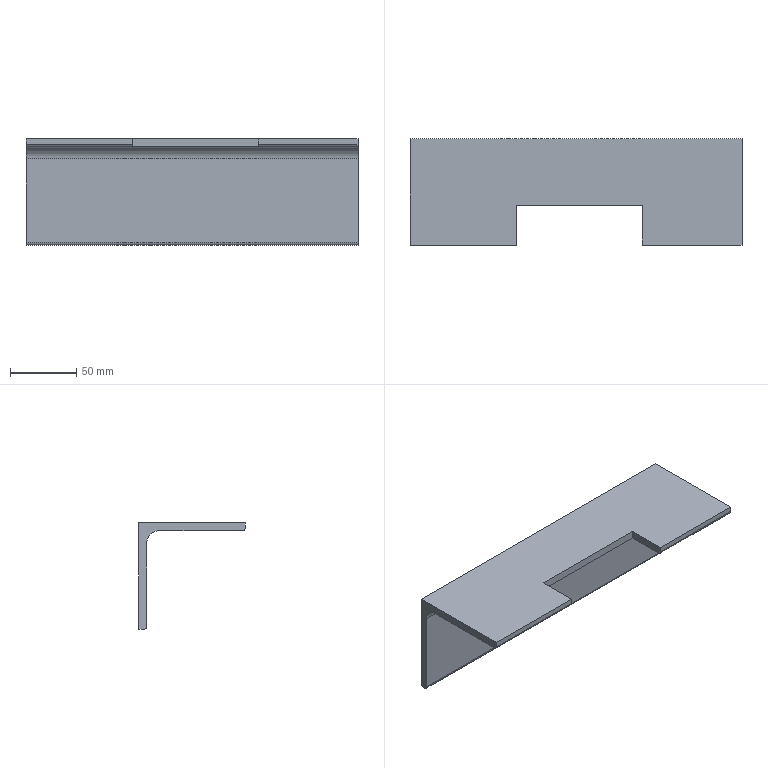Part | SolidWorks | features ICE 1, WeldMemberFeat 1, WeldmentFeature 1 | 1 solid | 16 faces | box 250 x 80 x 80 mm | volume 217898 mm3 | plane 12 | cylinder 4 | commonest cylinder face diameters 4 x3 18 x1
STEP:
#1=CARTESIAN_POINT('',(50.,-80.,0.));
#2=VERTEX_POINT('',#1);
#3=CARTESIAN_POINT('',(125.,-80.,0.));
#4=VERTEX_POINT('',#3);
#5=CARTESIAN_POINT('',(-125.,-80.,0.));
#6=DIRECTION('',(1.,0.,0.));
#7=VECTOR('',#6,1000.);
#8=LINE('',#5,#7);
#9=EDGE_CURVE('',#2,#4,#8,.T.);
#10=ORIENTED_EDGE('',*,*,#9,.F.);
#11=CARTESIAN_POINT('',(50.,-80.,-4.));
#12=VERTEX_POINT('',#11);
#13=CARTESIAN_POINT('',(50.,-80.,0.));
#14=DIRECTION('',(0.,0.,-1.));
#15=VECTOR('',#14,1000.);
#16=LINE('',#13,#15);
#17=EDGE_CURVE('',#2,#12,#16,.T.);
#18=ORIENTED_EDGE('',*,*,#17,.T.);
#19=CARTESIAN_POINT('',(125.,-80.,-4.));
#20=VERTEX_POINT('',#19);
#21=CARTESIAN_POINT('',(-125.,-80.,-4.));
#22=DIRECTION('',(1.,0.,0.));
#23=VECTOR('',#22,1000.);
#24=LINE('',#21,#23);
#25=EDGE_CURVE('',#12,#20,#24,.T.);
#26=ORIENTED_EDGE('',*,*,#25,.T.);
#27=CARTESIAN_POINT('',(125.,-80.,0.));
#28=DIRECTION('',(0.,0.,1.));
#29=VECTOR('',#28,1000.);
#30=LINE('',#27,#29);
#31=EDGE_CURVE('',#20,#4,#30,.T.);
#32=ORIENTED_EDGE('',*,*,#31,.T.);
#33=EDGE_LOOP('',(#10,#18,#26,#32));
#34=FACE_OUTER_BOUND('',#33,.T.);
#35=CARTESIAN_POINT('',(-125.,-80.,0.));
#36=DIRECTION('',(0.,1.,0.));
#37=DIRECTION('',(-1.,0.,0.));
#38=AXIS2_PLACEMENT_3D('',#35,#36,#37);
#39=PLANE('',#38);
#40=ADVANCED_FACE('',(#34),#39,.F.);
#41=ORIENTED_EDGE('',*,*,#25,.F.);
#42=CARTESIAN_POINT('',(50.,-78.,-6.));
#43=VERTEX_POINT('',#42);
#44=CARTESIAN_POINT('',(50.,-78.,-4.));
#45=DIRECTION('',(1.,0.,0.));
#46=DIRECTION('',(0.,1.,0.));
#47=AXIS2_PLACEMENT_3D('',#44,#45,#46);
#48=CIRCLE('',#47,2.);
#49=EDGE_CURVE('',#12,#43,#48,.T.);
#50=ORIENTED_EDGE('',*,*,#49,.T.);
#51=CARTESIAN_POINT('',(125.,-78.,-6.));
#52=VERTEX_POINT('',#51);
#53=CARTESIAN_POINT('',(-125.,-78.,-6.));
#54=DIRECTION('',(1.,0.,0.));
#55=VECTOR('',#54,1000.);
#56=LINE('',#53,#55);
#57=EDGE_CURVE('',#43,#52,#56,.T.);
#58=ORIENTED_EDGE('',*,*,#57,.T.);
#59=CARTESIAN_POINT('',(125.,-78.,-4.));
#60=DIRECTION('',(-1.,0.,0.));
#61=DIRECTION('',(0.,1.,0.));
#62=AXIS2_PLACEMENT_3D('',#59,#60,#61);
#63=CIRCLE('',#62,2.);
#64=EDGE_CURVE('',#52,#20,#63,.T.);
#65=ORIENTED_EDGE('',*,*,#64,.T.);
#66=EDGE_LOOP('',(#41,#50,#58,#65));
#67=FACE_OUTER_BOUND('',#66,.T.);
#68=CARTESIAN_POINT('',(-125.,-78.,-4.));
#69=DIRECTION('',(1.,0.,0.));
#70=DIRECTION('',(0.,1.,0.));
#71=AXIS2_PLACEMENT_3D('',#68,#69,#70);
#72=CYLINDRICAL_SURFACE('',#71,2.);
#73=ADVANCED_FACE('',(#67),#72,.T.);
#74=CARTESIAN_POINT('',(-125.,-80.,-4.));
#75=VERTEX_POINT('',#74);
#76=CARTESIAN_POINT('',(-45.,-80.,-4.));
#77=VERTEX_POINT('',#76);
#78=CARTESIAN_POINT('',(-125.,-80.,-4.));
#79=DIRECTION('',(1.,0.,0.));
#80=VECTOR('',#79,1000.);
#81=LINE('',#78,#80);
#82=EDGE_CURVE('',#75,#77,#81,.T.);
#83=ORIENTED_EDGE('',*,*,#82,.T.);
#84=CARTESIAN_POINT('',(-45.,-80.,0.));
#85=VERTEX_POINT('',#84);
#86=CARTESIAN_POINT('',(-45.,-80.,0.));
#87=DIRECTION('',(0.,0.,1.));
#88=VECTOR('',#87,1000.);
#89=LINE('',#86,#88);
#90=EDGE_CURVE('',#77,#85,#89,.T.);
#91=ORIENTED_EDGE('',*,*,#90,.T.);
#92=CARTESIAN_POINT('',(-125.,-80.,0.));
#93=VERTEX_POINT('',#92);
#94=CARTESIAN_POINT('',(-125.,-80.,0.));
#95=DIRECTION('',(1.,0.,0.));
#96=VECTOR('',#95,1000.);
#97=LINE('',#94,#96);
#98=EDGE_CURVE('',#93,#85,#97,.T.);
#99=ORIENTED_EDGE('',*,*,#98,.F.);
#100=CARTESIAN_POINT('',(-125.,-80.,0.));
#101=DIRECTION('',(0.,0.,1.));
#102=VECTOR('',#101,1000.);
#103=LINE('',#100,#102);
#104=EDGE_CURVE('',#75,#93,#103,.T.);
#105=ORIENTED_EDGE('',*,*,#104,.F.);
#106=EDGE_LOOP('',(#83,#91,#99,#105));
#107=FACE_OUTER_BOUND('',#106,.T.);
#108=CARTESIAN_POINT('',(-125.,-80.,0.));
#109=DIRECTION('',(0.,1.,0.));
#110=DIRECTION('',(-1.,0.,0.));
#111=AXIS2_PLACEMENT_3D('',#108,#109,#110);
#112=PLANE('',#111);
#113=ADVANCED_FACE('',(#107),#112,.F.);
#114=CARTESIAN_POINT('',(-45.,-50.,0.));
#115=VERTEX_POINT('',#114);
#116=CARTESIAN_POINT('',(50.,-50.,0.));
#117=VERTEX_POINT('',#116);
#118=CARTESIAN_POINT('',(-125.,-50.,0.));
#119=DIRECTION('',(1.,0.,0.));
#120=VECTOR('',#119,1000.);
#121=LINE('',#118,#120);
#122=EDGE_CURVE('',#115,#117,#121,.T.);
#123=ORIENTED_EDGE('',*,*,#122,.T.);
#124=CARTESIAN_POINT('',(50.,-80.,0.));
#125=DIRECTION('',(0.,-1.,0.));
#126=VECTOR('',#125,1000.);
#127=LINE('',#124,#126);
#128=EDGE_CURVE('',#117,#2,#127,.T.);
#129=ORIENTED_EDGE('',*,*,#128,.T.);
#130=ORIENTED_EDGE('',*,*,#9,.T.);
#131=CARTESIAN_POINT('',(125.,0.,0.));
#132=VERTEX_POINT('',#131);
#133=CARTESIAN_POINT('',(125.,-80.,0.));
#134=DIRECTION('',(0.,1.,0.));
#135=VECTOR('',#134,1000.);
#136=LINE('',#133,#135);
#137=EDGE_CURVE('',#4,#132,#136,.T.);
#138=ORIENTED_EDGE('',*,*,#137,.T.);
#139=CARTESIAN_POINT('',(-125.,0.,0.));
#140=VERTEX_POINT('',#139);
#141=CARTESIAN_POINT('',(-125.,0.,0.));
#142=DIRECTION('',(1.,0.,0.));
#143=VECTOR('',#142,1000.);
#144=LINE('',#141,#143);
#145=EDGE_CURVE('',#140,#132,#144,.T.);
#146=ORIENTED_EDGE('',*,*,#145,.F.);
#147=CARTESIAN_POINT('',(-125.,-80.,0.));
#148=DIRECTION('',(0.,1.,0.));
#149=VECTOR('',#148,1000.);
#150=LINE('',#147,#149);
#151=EDGE_CURVE('',#93,#140,#150,.T.);
#152=ORIENTED_EDGE('',*,*,#151,.F.);
#153=ORIENTED_EDGE('',*,*,#98,.T.);
#154=CARTESIAN_POINT('',(-45.,-80.,0.));
#155=DIRECTION('',(0.,1.,0.));
#156=VECTOR('',#155,1000.);
#157=LINE('',#154,#156);
#158=EDGE_CURVE('',#85,#115,#157,.T.);
#159=ORIENTED_EDGE('',*,*,#158,.T.);
#160=EDGE_LOOP('',(#123,#129,#130,#138,#146,#152,#153,#159));
#161=FACE_OUTER_BOUND('',#160,.T.);
#162=CARTESIAN_POINT('',(-125.,-80.,0.));
#163=DIRECTION('',(0.,0.,-1.));
#164=DIRECTION('',(0.,1.,0.));
#165=AXIS2_PLACEMENT_3D('',#162,#163,#164);
#166=PLANE('',#165);
#167=ADVANCED_FACE('',(#161),#166,.F.);
#168=CARTESIAN_POINT('',(125.,0.,-80.));
#169=VERTEX_POINT('',#168);
#170=CARTESIAN_POINT('',(125.,0.,0.));
#171=DIRECTION('',(0.,0.,-1.));
#172=VECTOR('',#171,1000.);
#173=LINE('',#170,#172);
#174=EDGE_CURVE('',#132,#169,#173,.T.);
#175=ORIENTED_EDGE('',*,*,#174,.T.);
#176=CARTESIAN_POINT('',(-125.,0.,-80.));
#177=VERTEX_POINT('',#176);
#178=CARTESIAN_POINT('',(-125.,0.,-80.));
#179=DIRECTION('',(1.,0.,0.));
#180=VECTOR('',#179,1000.);
#181=LINE('',#178,#180);
#182=EDGE_CURVE('',#177,#169,#181,.T.);
#183=ORIENTED_EDGE('',*,*,#182,.F.);
#184=CARTESIAN_POINT('',(-125.,0.,0.));
#185=DIRECTION('',(0.,0.,-1.));
#186=VECTOR('',#185,1000.);
#187=LINE('',#184,#186);
#188=EDGE_CURVE('',#140,#177,#187,.T.);
#189=ORIENTED_EDGE('',*,*,#188,.F.);
#190=ORIENTED_EDGE('',*,*,#145,.T.);
#191=EDGE_LOOP('',(#175,#183,#189,#190));
#192=FACE_OUTER_BOUND('',#191,.T.);
#193=CARTESIAN_POINT('',(-125.,0.,0.));
#194=DIRECTION('',(0.,-1.,0.));
#195=DIRECTION('',(1.,0.,0.));
#196=AXIS2_PLACEMENT_3D('',#193,#194,#195);
#197=PLANE('',#196);
#198=ADVANCED_FACE('',(#192),#197,.F.);
#199=CARTESIAN_POINT('',(125.,-4.,-80.));
#200=VERTEX_POINT('',#199);
#201=CARTESIAN_POINT('',(125.,0.,-80.));
#202=DIRECTION('',(0.,-1.,0.));
#203=VECTOR('',#202,1000.);
#204=LINE('',#201,#203);
#205=EDGE_CURVE('',#169,#200,#204,.T.);
#206=ORIENTED_EDGE('',*,*,#205,.T.);
#207=CARTESIAN_POINT('',(-125.,-4.,-80.));
#208=VERTEX_POINT('',#207);
#209=CARTESIAN_POINT('',(-125.,-4.,-80.));
#210=DIRECTION('',(1.,0.,0.));
#211=VECTOR('',#210,1000.);
#212=LINE('',#209,#211);
#213=EDGE_CURVE('',#208,#200,#212,.T.);
#214=ORIENTED_EDGE('',*,*,#213,.F.);
#215=CARTESIAN_POINT('',(-125.,0.,-80.));
#216=DIRECTION('',(0.,-1.,0.));
#217=VECTOR('',#216,1000.);
#218=LINE('',#215,#217);
#219=EDGE_CURVE('',#177,#208,#218,.T.);
#220=ORIENTED_EDGE('',*,*,#219,.F.);
#221=ORIENTED_EDGE('',*,*,#182,.T.);
#222=EDGE_LOOP('',(#206,#214,#220,#221));
#223=FACE_OUTER_BOUND('',#222,.T.);
#224=CARTESIAN_POINT('',(-125.,0.,-80.));
#225=DIRECTION('',(0.,0.,1.));
#226=DIRECTION('',(0.,-1.,0.));
#227=AXIS2_PLACEMENT_3D('',#224,#225,#226);
#228=PLANE('',#227);
#229=ADVANCED_FACE('',(#223),#228,.F.);
#230=CARTESIAN_POINT('',(125.,-6.,-78.));
#231=VERTEX_POINT('',#230);
#232=CARTESIAN_POINT('',(125.,-4.,-78.));
#233=DIRECTION('',(-1.,0.,0.));
#234=DIRECTION('',(0.,-1.,0.));
#235=AXIS2_PLACEMENT_3D('',#232,#233,#234);
#236=CIRCLE('',#235,2.);
#237=EDGE_CURVE('',#200,#231,#236,.T.);
#238=ORIENTED_EDGE('',*,*,#237,.T.);
#239=CARTESIAN_POINT('',(-125.,-6.,-78.));
#240=VERTEX_POINT('',#239);
#241=CARTESIAN_POINT('',(-125.,-6.,-78.));
#242=DIRECTION('',(1.,0.,0.));
#243=VECTOR('',#242,1000.);
#244=LINE('',#241,#243);
#245=EDGE_CURVE('',#240,#231,#244,.T.);
#246=ORIENTED_EDGE('',*,*,#245,.F.);
#247=CARTESIAN_POINT('',(-125.,-4.,-78.));
#248=DIRECTION('',(-1.,0.,0.));
#249=DIRECTION('',(0.,-1.,0.));
#250=AXIS2_PLACEMENT_3D('',#247,#248,#249);
#251=CIRCLE('',#250,2.);
#252=EDGE_CURVE('',#208,#240,#251,.T.);
#253=ORIENTED_EDGE('',*,*,#252,.F.);
#254=ORIENTED_EDGE('',*,*,#213,.T.);
#255=EDGE_LOOP('',(#238,#246,#253,#254));
#256=FACE_OUTER_BOUND('',#255,.T.);
#257=CARTESIAN_POINT('',(-125.,-4.,-78.));
#258=DIRECTION('',(1.,0.,0.));
#259=DIRECTION('',(0.,1.,0.));
#260=AXIS2_PLACEMENT_3D('',#257,#258,#259);
#261=CYLINDRICAL_SURFACE('',#260,2.);
#262=ADVANCED_FACE('',(#256),#261,.T.);
#263=CARTESIAN_POINT('',(125.,-6.,-15.));
#264=VERTEX_POINT('',#263);
#265=CARTESIAN_POINT('',(125.,-6.,-15.));
#266=DIRECTION('',(0.,0.,1.));
#267=VECTOR('',#266,1000.);
#268=LINE('',#265,#267);
#269=EDGE_CURVE('',#231,#264,#268,.T.);
#270=ORIENTED_EDGE('',*,*,#269,.T.);
#271=CARTESIAN_POINT('',(-125.,-6.,-15.));
#272=VERTEX_POINT('',#271);
#273=CARTESIAN_POINT('',(-125.,-6.,-15.));
#274=DIRECTION('',(1.,0.,0.));
#275=VECTOR('',#274,1000.);
#276=LINE('',#273,#275);
#277=EDGE_CURVE('',#272,#264,#276,.T.);
#278=ORIENTED_EDGE('',*,*,#277,.F.);
#279=CARTESIAN_POINT('',(-125.,-6.,-15.));
#280=DIRECTION('',(0.,0.,1.));
#281=VECTOR('',#280,1000.);
#282=LINE('',#279,#281);
#283=EDGE_CURVE('',#240,#272,#282,.T.);
#284=ORIENTED_EDGE('',*,*,#283,.F.);
#285=ORIENTED_EDGE('',*,*,#245,.T.);
#286=EDGE_LOOP('',(#270,#278,#284,#285));
#287=FACE_OUTER_BOUND('',#286,.T.);
#288=CARTESIAN_POINT('',(-125.,-6.,-15.));
#289=DIRECTION('',(0.,1.,0.));
#290=DIRECTION('',(-1.,0.,0.));
#291=AXIS2_PLACEMENT_3D('',#288,#289,#290);
#292=PLANE('',#291);
#293=ADVANCED_FACE('',(#287),#292,.F.);
#294=CARTESIAN_POINT('',(125.,-15.,-6.));
#295=VERTEX_POINT('',#294);
#296=CARTESIAN_POINT('',(125.,-15.,-15.));
#297=DIRECTION('',(1.,0.,0.));
#298=DIRECTION('',(0.,-1.,0.));
#299=AXIS2_PLACEMENT_3D('',#296,#297,#298);
#300=CIRCLE('',#299,9.);
#301=EDGE_CURVE('',#264,#295,#300,.T.);
#302=ORIENTED_EDGE('',*,*,#301,.T.);
#303=CARTESIAN_POINT('',(-125.,-15.,-6.));
#304=VERTEX_POINT('',#303);
#305=CARTESIAN_POINT('',(-125.,-15.,-6.));
#306=DIRECTION('',(1.,0.,0.));
#307=VECTOR('',#306,1000.);
#308=LINE('',#305,#307);
#309=EDGE_CURVE('',#304,#295,#308,.T.);
#310=ORIENTED_EDGE('',*,*,#309,.F.);
#311=CARTESIAN_POINT('',(-125.,-15.,-15.));
#312=DIRECTION('',(1.,0.,0.));
#313=DIRECTION('',(0.,-1.,0.));
#314=AXIS2_PLACEMENT_3D('',#311,#312,#313);
#315=CIRCLE('',#314,9.);
#316=EDGE_CURVE('',#272,#304,#315,.T.);
#317=ORIENTED_EDGE('',*,*,#316,.F.);
#318=ORIENTED_EDGE('',*,*,#277,.T.);
#319=EDGE_LOOP('',(#302,#310,#317,#318));
#320=FACE_OUTER_BOUND('',#319,.T.);
#321=CARTESIAN_POINT('',(-125.,-15.,-15.));
#322=DIRECTION('',(1.,0.,0.));
#323=DIRECTION('',(0.,1.,0.));
#324=AXIS2_PLACEMENT_3D('',#321,#322,#323);
#325=CYLINDRICAL_SURFACE('',#324,9.);
#326=ADVANCED_FACE('',(#320),#325,.F.);
#327=ORIENTED_EDGE('',*,*,#57,.F.);
#328=CARTESIAN_POINT('',(50.,-50.,-6.));
#329=VERTEX_POINT('',#328);
#330=CARTESIAN_POINT('',(50.,-50.,-6.));
#331=DIRECTION('',(0.,-1.,0.));
#332=VECTOR('',#331,1000.);
#333=LINE('',#330,#332);
#334=EDGE_CURVE('',#329,#43,#333,.T.);
#335=ORIENTED_EDGE('',*,*,#334,.F.);
#336=CARTESIAN_POINT('',(-45.,-50.,-6.));
#337=VERTEX_POINT('',#336);
#338=CARTESIAN_POINT('',(-45.,-50.,-6.));
#339=DIRECTION('',(1.,0.,0.));
#340=VECTOR('',#339,1000.);
#341=LINE('',#338,#340);
#342=EDGE_CURVE('',#337,#329,#341,.T.);
#343=ORIENTED_EDGE('',*,*,#342,.F.);
#344=CARTESIAN_POINT('',(-45.,-78.,-6.));
#345=VERTEX_POINT('',#344);
#346=CARTESIAN_POINT('',(-45.,-99.52,-6.));
#347=DIRECTION('',(0.,1.,0.));
#348=VECTOR('',#347,1000.);
#349=LINE('',#346,#348);
#350=EDGE_CURVE('',#345,#337,#349,.T.);
#351=ORIENTED_EDGE('',*,*,#350,.F.);
#352=CARTESIAN_POINT('',(-125.,-78.,-6.));
#353=VERTEX_POINT('',#352);
#354=CARTESIAN_POINT('',(-125.,-78.,-6.));
#355=DIRECTION('',(1.,0.,0.));
#356=VECTOR('',#355,1000.);
#357=LINE('',#354,#356);
#358=EDGE_CURVE('',#353,#345,#357,.T.);
#359=ORIENTED_EDGE('',*,*,#358,.F.);
#360=CARTESIAN_POINT('',(-125.,-78.,-6.));
#361=DIRECTION('',(0.,-1.,0.));
#362=VECTOR('',#361,1000.);
#363=LINE('',#360,#362);
#364=EDGE_CURVE('',#304,#353,#363,.T.);
#365=ORIENTED_EDGE('',*,*,#364,.F.);
#366=ORIENTED_EDGE('',*,*,#309,.T.);
#367=CARTESIAN_POINT('',(125.,-78.,-6.));
#368=DIRECTION('',(0.,-1.,0.));
#369=VECTOR('',#368,1000.);
#370=LINE('',#367,#369);
#371=EDGE_CURVE('',#295,#52,#370,.T.);
#372=ORIENTED_EDGE('',*,*,#371,.T.);
#373=EDGE_LOOP('',(#327,#335,#343,#351,#359,#365,#366,#372));
#374=FACE_OUTER_BOUND('',#373,.T.);
#375=CARTESIAN_POINT('',(-125.,-78.,-6.));
#376=DIRECTION('',(0.,0.,1.));
#377=DIRECTION('',(0.,-1.,0.));
#378=AXIS2_PLACEMENT_3D('',#375,#376,#377);
#379=PLANE('',#378);
#380=ADVANCED_FACE('',(#374),#379,.F.);
#381=ORIENTED_EDGE('',*,*,#358,.T.);
#382=CARTESIAN_POINT('',(-45.,-78.,-4.));
#383=DIRECTION('',(-1.,0.,0.));
#384=DIRECTION('',(0.,0.,1.));
#385=AXIS2_PLACEMENT_3D('',#382,#383,#384);
#386=CIRCLE('',#385,2.);
#387=EDGE_CURVE('',#345,#77,#386,.T.);
#388=ORIENTED_EDGE('',*,*,#387,.T.);
#389=ORIENTED_EDGE('',*,*,#82,.F.);
#390=CARTESIAN_POINT('',(-125.,-78.,-4.));
#391=DIRECTION('',(-1.,0.,0.));
#392=DIRECTION('',(0.,1.,0.));
#393=AXIS2_PLACEMENT_3D('',#390,#391,#392);
#394=CIRCLE('',#393,2.);
#395=EDGE_CURVE('',#353,#75,#394,.T.);
#396=ORIENTED_EDGE('',*,*,#395,.F.);
#397=EDGE_LOOP('',(#381,#388,#389,#396));
#398=FACE_OUTER_BOUND('',#397,.T.);
#399=CARTESIAN_POINT('',(-125.,-78.,-4.));
#400=DIRECTION('',(1.,0.,0.));
#401=DIRECTION('',(0.,1.,0.));
#402=AXIS2_PLACEMENT_3D('',#399,#400,#401);
#403=CYLINDRICAL_SURFACE('',#402,2.);
#404=ADVANCED_FACE('',(#398),#403,.T.);
#405=ORIENTED_EDGE('',*,*,#104,.T.);
#406=ORIENTED_EDGE('',*,*,#151,.T.);
#407=ORIENTED_EDGE('',*,*,#188,.T.);
#408=ORIENTED_EDGE('',*,*,#219,.T.);
#409=ORIENTED_EDGE('',*,*,#252,.T.);
#410=ORIENTED_EDGE('',*,*,#283,.T.);
#411=ORIENTED_EDGE('',*,*,#316,.T.);
#412=ORIENTED_EDGE('',*,*,#364,.T.);
#413=ORIENTED_EDGE('',*,*,#395,.T.);
#414=EDGE_LOOP('',(#405,#406,#407,#408,#409,#410,#411,#412,#413));
#415=FACE_OUTER_BOUND('',#414,.T.);
#416=CARTESIAN_POINT('',(-125.,-78.,-4.));
#417=DIRECTION('',(1.,0.,0.));
#418=DIRECTION('',(0.,1.,0.));
#419=AXIS2_PLACEMENT_3D('',#416,#417,#418);
#420=PLANE('',#419);
#421=ADVANCED_FACE('',(#415),#420,.F.);
#422=ORIENTED_EDGE('',*,*,#31,.F.);
#423=ORIENTED_EDGE('',*,*,#64,.F.);
#424=ORIENTED_EDGE('',*,*,#371,.F.);
#425=ORIENTED_EDGE('',*,*,#301,.F.);
#426=ORIENTED_EDGE('',*,*,#269,.F.);
#427=ORIENTED_EDGE('',*,*,#237,.F.);
#428=ORIENTED_EDGE('',*,*,#205,.F.);
#429=ORIENTED_EDGE('',*,*,#174,.F.);
#430=ORIENTED_EDGE('',*,*,#137,.F.);
#431=EDGE_LOOP('',(#422,#423,#424,#425,#426,#427,#428,#429,#430));
#432=FACE_OUTER_BOUND('',#431,.T.);
#433=CARTESIAN_POINT('',(125.,-78.,-4.));
#434=DIRECTION('',(1.,0.,0.));
#435=DIRECTION('',(0.,1.,0.));
#436=AXIS2_PLACEMENT_3D('',#433,#434,#435);
#437=PLANE('',#436);
#438=ADVANCED_FACE('',(#432),#437,.T.);
#439=CARTESIAN_POINT('',(-45.,-50.,4.));
#440=DIRECTION('',(0.,0.,-1.));
#441=VECTOR('',#440,1000.);
#442=LINE('',#439,#441);
#443=EDGE_CURVE('',#115,#337,#442,.T.);
#444=ORIENTED_EDGE('',*,*,#443,.T.);
#445=ORIENTED_EDGE('',*,*,#342,.T.);
#446=CARTESIAN_POINT('',(50.,-50.,4.));
#447=DIRECTION('',(0.,0.,-1.));
#448=VECTOR('',#447,1000.);
#449=LINE('',#446,#448);
#450=EDGE_CURVE('',#117,#329,#449,.T.);
#451=ORIENTED_EDGE('',*,*,#450,.F.);
#452=ORIENTED_EDGE('',*,*,#122,.F.);
#453=EDGE_LOOP('',(#444,#445,#451,#452));
#454=FACE_OUTER_BOUND('',#453,.T.);
#455=CARTESIAN_POINT('',(-45.,-50.,4.));
#456=DIRECTION('',(0.,1.,0.));
#457=DIRECTION('',(-1.,0.,0.));
#458=AXIS2_PLACEMENT_3D('',#455,#456,#457);
#459=PLANE('',#458);
#460=ADVANCED_FACE('',(#454),#459,.F.);
#461=ORIENTED_EDGE('',*,*,#450,.T.);
#462=ORIENTED_EDGE('',*,*,#334,.T.);
#463=ORIENTED_EDGE('',*,*,#49,.F.);
#464=ORIENTED_EDGE('',*,*,#17,.F.);
#465=ORIENTED_EDGE('',*,*,#128,.F.);
#466=EDGE_LOOP('',(#461,#462,#463,#464,#465));
#467=FACE_OUTER_BOUND('',#466,.T.);
#468=CARTESIAN_POINT('',(50.,-50.,4.));
#469=DIRECTION('',(1.,0.,0.));
#470=DIRECTION('',(0.,1.,0.));
#471=AXIS2_PLACEMENT_3D('',#468,#469,#470);
#472=PLANE('',#471);
#473=ADVANCED_FACE('',(#467),#472,.F.);
#474=ORIENTED_EDGE('',*,*,#90,.F.);
#475=ORIENTED_EDGE('',*,*,#387,.F.);
#476=ORIENTED_EDGE('',*,*,#350,.T.);
#477=ORIENTED_EDGE('',*,*,#443,.F.);
#478=ORIENTED_EDGE('',*,*,#158,.F.);
#479=EDGE_LOOP('',(#474,#475,#476,#477,#478));
#480=FACE_OUTER_BOUND('',#479,.T.);
#481=CARTESIAN_POINT('',(-45.,-99.52,4.));
#482=DIRECTION('',(-1.,0.,0.));
#483=DIRECTION('',(0.,0.,1.));
#484=AXIS2_PLACEMENT_3D('',#481,#482,#483);
#485=PLANE('',#484);
#486=ADVANCED_FACE('',(#480),#485,.F.);
#487=CLOSED_SHELL('',(#40,#73,#113,#167,#198,#229,#262,#293,#326,#380,#404,#421,#438,#460,#473,#486));
#488=MANIFOLD_SOLID_BREP('',#487);
#489=CARTESIAN_POINT('',(0.,0.,0.));
#490=DIRECTION('',(0.,0.,1.));
#491=DIRECTION('',(1.,0.,0.));
#492=AXIS2_PLACEMENT_3D('',#489,#490,#491);
#493=(LENGTH_UNIT()NAMED_UNIT(*)SI_UNIT(.MILLI.,.METRE.));
#494=UNCERTAINTY_MEASURE_WITH_UNIT(LENGTH_MEASURE(0.00001),#493,'','');
#495=(NAMED_UNIT(*)PLANE_ANGLE_UNIT()SI_UNIT($,.RADIAN.));
#496=(NAMED_UNIT(*)SI_UNIT($,.STERADIAN.)SOLID_ANGLE_UNIT());
#497=(GEOMETRIC_REPRESENTATION_CONTEXT(3)GLOBAL_UNCERTAINTY_ASSIGNED_CONTEXT((#494))GLOBAL_UNIT_ASSIGNED_CONTEXT((#493,#495,#496))REPRESENTATION_CONTEXT('',''));
#498=ADVANCED_BREP_SHAPE_REPRESENTATION('',(#488,#492),#497);